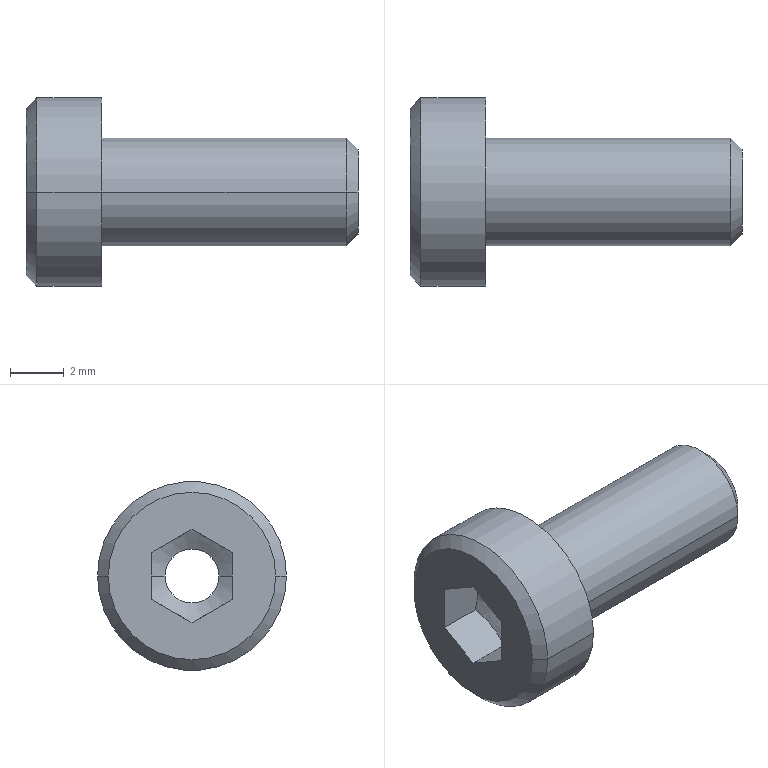Part | STEP file | ASND-0110-Solid1-1 | 1 solid | 21 faces | box 12.3 x 7 x 7 mm | volume 177.16 mm3 | plane 9 | cylinder 6 | cone 6 | commonest cylinder face diameters 2 x2 4 x2 7 x2